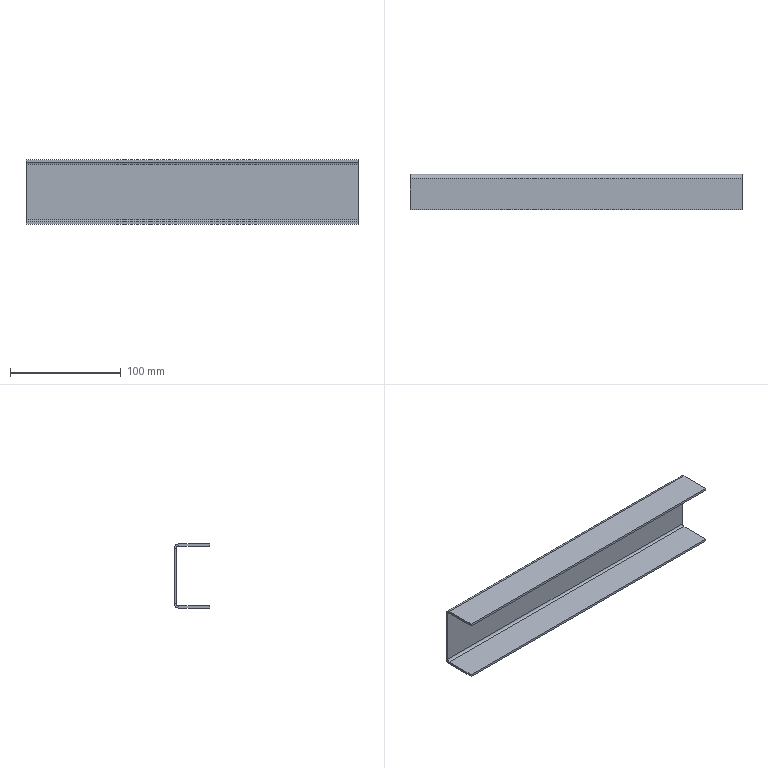Part | STEP file | JBJ-P-1007-04 | 1 solid | 22 faces | box 300 x 32 x 58 mm | volume 69255 mm3 | plane 18 | cylinder 4 | commonest cylinder face diameters 4 x2 8 x2
STEP:
#1=CARTESIAN_POINT('',(300.,28.,0.));
#2=VERTEX_POINT('',#1);
#3=CARTESIAN_POINT('',(300.,28.,2.));
#4=VERTEX_POINT('',#3);
#5=CARTESIAN_POINT('',(300.,28.,0.));
#6=DIRECTION('',(0.,0.,1.));
#7=VECTOR('',#6,1000.);
#8=LINE('',#5,#7);
#9=EDGE_CURVE('',#2,#4,#8,.T.);
#10=ORIENTED_EDGE('',*,*,#9,.F.);
#11=CARTESIAN_POINT('',(300.,30.,-2.));
#12=VERTEX_POINT('',#11);
#13=CARTESIAN_POINT('',(300.,28.,-2.));
#14=DIRECTION('',(-1.,0.,0.));
#15=DIRECTION('',(0.,0.,-1.));
#16=AXIS2_PLACEMENT_3D('',#13,#14,#15);
#17=CIRCLE('',#16,2.);
#18=EDGE_CURVE('',#2,#12,#17,.T.);
#19=ORIENTED_EDGE('',*,*,#18,.T.);
#20=CARTESIAN_POINT('',(300.,32.,-2.));
#21=VERTEX_POINT('',#20);
#22=CARTESIAN_POINT('',(300.,32.,-2.));
#23=DIRECTION('',(0.,-1.,0.));
#24=VECTOR('',#23,1000.);
#25=LINE('',#22,#24);
#26=EDGE_CURVE('',#21,#12,#25,.T.);
#27=ORIENTED_EDGE('',*,*,#26,.F.);
#28=CARTESIAN_POINT('',(300.,28.,-2.));
#29=DIRECTION('',(-1.,0.,0.));
#30=DIRECTION('',(0.,0.,-1.));
#31=AXIS2_PLACEMENT_3D('',#28,#29,#30);
#32=CIRCLE('',#31,4.);
#33=EDGE_CURVE('',#4,#21,#32,.T.);
#34=ORIENTED_EDGE('',*,*,#33,.F.);
#35=EDGE_LOOP('',(#10,#19,#27,#34));
#36=FACE_OUTER_BOUND('',#35,.T.);
#37=CARTESIAN_POINT('',(300.,28.,0.));
#38=DIRECTION('',(1.,0.,0.));
#39=DIRECTION('',(0.,0.,-1.));
#40=AXIS2_PLACEMENT_3D('',#37,#38,#39);
#41=PLANE('',#40);
#42=ADVANCED_FACE('',(#36),#41,.T.);
#43=CARTESIAN_POINT('',(300.,0.,0.));
#44=VERTEX_POINT('',#43);
#45=CARTESIAN_POINT('',(300.,0.,0.));
#46=DIRECTION('',(0.,1.,0.));
#47=VECTOR('',#46,1000.);
#48=LINE('',#45,#47);
#49=EDGE_CURVE('',#44,#2,#48,.T.);
#50=ORIENTED_EDGE('',*,*,#49,.T.);
#51=ORIENTED_EDGE('',*,*,#9,.T.);
#52=CARTESIAN_POINT('',(300.,0.,2.));
#53=VERTEX_POINT('',#52);
#54=CARTESIAN_POINT('',(300.,0.,2.));
#55=DIRECTION('',(0.,1.,0.));
#56=VECTOR('',#55,1000.);
#57=LINE('',#54,#56);
#58=EDGE_CURVE('',#53,#4,#57,.T.);
#59=ORIENTED_EDGE('',*,*,#58,.F.);
#60=CARTESIAN_POINT('',(300.,0.,0.));
#61=DIRECTION('',(0.,0.,1.));
#62=VECTOR('',#61,1000.);
#63=LINE('',#60,#62);
#64=EDGE_CURVE('',#44,#53,#63,.T.);
#65=ORIENTED_EDGE('',*,*,#64,.F.);
#66=EDGE_LOOP('',(#50,#51,#59,#65));
#67=FACE_OUTER_BOUND('',#66,.T.);
#68=CARTESIAN_POINT('',(300.,32.,-2.));
#69=DIRECTION('',(1.,0.,0.));
#70=DIRECTION('',(0.,0.,-1.));
#71=AXIS2_PLACEMENT_3D('',#68,#69,#70);
#72=PLANE('',#71);
#73=ADVANCED_FACE('',(#67),#72,.T.);
#74=CARTESIAN_POINT('',(0.,30.,-2.));
#75=VERTEX_POINT('',#74);
#76=CARTESIAN_POINT('',(0.,32.,-2.));
#77=VERTEX_POINT('',#76);
#78=CARTESIAN_POINT('',(0.,30.,-2.));
#79=DIRECTION('',(0.,1.,0.));
#80=VECTOR('',#79,1000.);
#81=LINE('',#78,#80);
#82=EDGE_CURVE('',#75,#77,#81,.T.);
#83=ORIENTED_EDGE('',*,*,#82,.F.);
#84=CARTESIAN_POINT('',(0.,28.,0.));
#85=VERTEX_POINT('',#84);
#86=CARTESIAN_POINT('',(0.,28.,-2.));
#87=DIRECTION('',(-1.,0.,0.));
#88=DIRECTION('',(0.,0.,-1.));
#89=AXIS2_PLACEMENT_3D('',#86,#87,#88);
#90=CIRCLE('',#89,2.);
#91=EDGE_CURVE('',#85,#75,#90,.T.);
#92=ORIENTED_EDGE('',*,*,#91,.F.);
#93=CARTESIAN_POINT('',(0.,28.,2.));
#94=VERTEX_POINT('',#93);
#95=CARTESIAN_POINT('',(0.,28.,2.));
#96=DIRECTION('',(0.,0.,-1.));
#97=VECTOR('',#96,1000.);
#98=LINE('',#95,#97);
#99=EDGE_CURVE('',#94,#85,#98,.T.);
#100=ORIENTED_EDGE('',*,*,#99,.F.);
#101=CARTESIAN_POINT('',(0.,28.,-2.));
#102=DIRECTION('',(-1.,0.,0.));
#103=DIRECTION('',(0.,0.,-1.));
#104=AXIS2_PLACEMENT_3D('',#101,#102,#103);
#105=CIRCLE('',#104,4.);
#106=EDGE_CURVE('',#94,#77,#105,.T.);
#107=ORIENTED_EDGE('',*,*,#106,.T.);
#108=EDGE_LOOP('',(#83,#92,#100,#107));
#109=FACE_OUTER_BOUND('',#108,.T.);
#110=CARTESIAN_POINT('',(0.,30.,-2.));
#111=DIRECTION('',(-1.,0.,0.));
#112=DIRECTION('',(0.,0.,1.));
#113=AXIS2_PLACEMENT_3D('',#110,#111,#112);
#114=PLANE('',#113);
#115=ADVANCED_FACE('',(#109),#114,.T.);
#116=CARTESIAN_POINT('',(0.,30.,-52.));
#117=VERTEX_POINT('',#116);
#118=CARTESIAN_POINT('',(0.,30.,0.));
#119=DIRECTION('',(0.,0.,-1.));
#120=VECTOR('',#119,1000.);
#121=LINE('',#118,#120);
#122=EDGE_CURVE('',#75,#117,#121,.T.);
#123=ORIENTED_EDGE('',*,*,#122,.F.);
#124=ORIENTED_EDGE('',*,*,#82,.T.);
#125=CARTESIAN_POINT('',(0.,32.,-52.));
#126=VERTEX_POINT('',#125);
#127=CARTESIAN_POINT('',(0.,32.,0.));
#128=DIRECTION('',(0.,0.,-1.));
#129=VECTOR('',#128,1000.);
#130=LINE('',#127,#129);
#131=EDGE_CURVE('',#77,#126,#130,.T.);
#132=ORIENTED_EDGE('',*,*,#131,.T.);
#133=CARTESIAN_POINT('',(0.,32.,-52.));
#134=DIRECTION('',(0.,-1.,0.));
#135=VECTOR('',#134,1000.);
#136=LINE('',#133,#135);
#137=EDGE_CURVE('',#126,#117,#136,.T.);
#138=ORIENTED_EDGE('',*,*,#137,.T.);
#139=EDGE_LOOP('',(#123,#124,#132,#138));
#140=FACE_OUTER_BOUND('',#139,.T.);
#141=CARTESIAN_POINT('',(0.,28.,2.));
#142=DIRECTION('',(-1.,0.,0.));
#143=DIRECTION('',(0.,0.,1.));
#144=AXIS2_PLACEMENT_3D('',#141,#142,#143);
#145=PLANE('',#144);
#146=ADVANCED_FACE('',(#140),#145,.T.);
#147=CARTESIAN_POINT('',(300.,30.,-52.));
#148=VERTEX_POINT('',#147);
#149=CARTESIAN_POINT('',(300.,32.,-52.));
#150=VERTEX_POINT('',#149);
#151=CARTESIAN_POINT('',(300.,30.,-52.));
#152=DIRECTION('',(0.,1.,0.));
#153=VECTOR('',#152,1000.);
#154=LINE('',#151,#153);
#155=EDGE_CURVE('',#148,#150,#154,.T.);
#156=ORIENTED_EDGE('',*,*,#155,.F.);
#157=CARTESIAN_POINT('',(300.,28.,-54.));
#158=VERTEX_POINT('',#157);
#159=CARTESIAN_POINT('',(300.,28.,-52.));
#160=DIRECTION('',(-1.,0.,0.));
#161=DIRECTION('',(0.,0.,-1.));
#162=AXIS2_PLACEMENT_3D('',#159,#160,#161);
#163=CIRCLE('',#162,2.);
#164=EDGE_CURVE('',#148,#158,#163,.T.);
#165=ORIENTED_EDGE('',*,*,#164,.T.);
#166=CARTESIAN_POINT('',(300.,28.,-56.));
#167=VERTEX_POINT('',#166);
#168=CARTESIAN_POINT('',(300.,28.,-56.));
#169=DIRECTION('',(0.,0.,1.));
#170=VECTOR('',#169,1000.);
#171=LINE('',#168,#170);
#172=EDGE_CURVE('',#167,#158,#171,.T.);
#173=ORIENTED_EDGE('',*,*,#172,.F.);
#174=CARTESIAN_POINT('',(300.,28.,-52.));
#175=DIRECTION('',(-1.,0.,0.));
#176=DIRECTION('',(0.,0.,-1.));
#177=AXIS2_PLACEMENT_3D('',#174,#175,#176);
#178=CIRCLE('',#177,4.);
#179=EDGE_CURVE('',#150,#167,#178,.T.);
#180=ORIENTED_EDGE('',*,*,#179,.F.);
#181=EDGE_LOOP('',(#156,#165,#173,#180));
#182=FACE_OUTER_BOUND('',#181,.T.);
#183=CARTESIAN_POINT('',(300.,30.,-52.));
#184=DIRECTION('',(1.,0.,0.));
#185=DIRECTION('',(0.,0.,-1.));
#186=AXIS2_PLACEMENT_3D('',#183,#184,#185);
#187=PLANE('',#186);
#188=ADVANCED_FACE('',(#182),#187,.T.);
#189=CARTESIAN_POINT('',(300.,30.,0.));
#190=DIRECTION('',(0.,0.,-1.));
#191=VECTOR('',#190,1000.);
#192=LINE('',#189,#191);
#193=EDGE_CURVE('',#12,#148,#192,.T.);
#194=ORIENTED_EDGE('',*,*,#193,.T.);
#195=ORIENTED_EDGE('',*,*,#155,.T.);
#196=CARTESIAN_POINT('',(300.,32.,0.));
#197=DIRECTION('',(0.,0.,-1.));
#198=VECTOR('',#197,1000.);
#199=LINE('',#196,#198);
#200=EDGE_CURVE('',#21,#150,#199,.T.);
#201=ORIENTED_EDGE('',*,*,#200,.F.);
#202=ORIENTED_EDGE('',*,*,#26,.T.);
#203=EDGE_LOOP('',(#194,#195,#201,#202));
#204=FACE_OUTER_BOUND('',#203,.T.);
#205=CARTESIAN_POINT('',(300.,28.,-56.));
#206=DIRECTION('',(1.,0.,0.));
#207=DIRECTION('',(0.,0.,-1.));
#208=AXIS2_PLACEMENT_3D('',#205,#206,#207);
#209=PLANE('',#208);
#210=ADVANCED_FACE('',(#204),#209,.T.);
#211=CARTESIAN_POINT('',(0.,28.,-54.));
#212=VERTEX_POINT('',#211);
#213=CARTESIAN_POINT('',(0.,28.,-56.));
#214=VERTEX_POINT('',#213);
#215=CARTESIAN_POINT('',(0.,28.,-54.));
#216=DIRECTION('',(0.,0.,-1.));
#217=VECTOR('',#216,1000.);
#218=LINE('',#215,#217);
#219=EDGE_CURVE('',#212,#214,#218,.T.);
#220=ORIENTED_EDGE('',*,*,#219,.F.);
#221=CARTESIAN_POINT('',(0.,28.,-52.));
#222=DIRECTION('',(-1.,0.,0.));
#223=DIRECTION('',(0.,0.,-1.));
#224=AXIS2_PLACEMENT_3D('',#221,#222,#223);
#225=CIRCLE('',#224,2.);
#226=EDGE_CURVE('',#117,#212,#225,.T.);
#227=ORIENTED_EDGE('',*,*,#226,.F.);
#228=ORIENTED_EDGE('',*,*,#137,.F.);
#229=CARTESIAN_POINT('',(0.,28.,-52.));
#230=DIRECTION('',(-1.,0.,0.));
#231=DIRECTION('',(0.,0.,-1.));
#232=AXIS2_PLACEMENT_3D('',#229,#230,#231);
#233=CIRCLE('',#232,4.);
#234=EDGE_CURVE('',#126,#214,#233,.T.);
#235=ORIENTED_EDGE('',*,*,#234,.T.);
#236=EDGE_LOOP('',(#220,#227,#228,#235));
#237=FACE_OUTER_BOUND('',#236,.T.);
#238=CARTESIAN_POINT('',(0.,28.,-54.));
#239=DIRECTION('',(-1.,0.,0.));
#240=DIRECTION('',(0.,0.,1.));
#241=AXIS2_PLACEMENT_3D('',#238,#239,#240);
#242=PLANE('',#241);
#243=ADVANCED_FACE('',(#237),#242,.T.);
#244=CARTESIAN_POINT('',(0.,0.,-54.));
#245=VERTEX_POINT('',#244);
#246=CARTESIAN_POINT('',(0.,30.,-54.));
#247=DIRECTION('',(0.,-1.,0.));
#248=VECTOR('',#247,1000.);
#249=LINE('',#246,#248);
#250=EDGE_CURVE('',#212,#245,#249,.T.);
#251=ORIENTED_EDGE('',*,*,#250,.F.);
#252=ORIENTED_EDGE('',*,*,#219,.T.);
#253=CARTESIAN_POINT('',(0.,0.,-56.));
#254=VERTEX_POINT('',#253);
#255=CARTESIAN_POINT('',(0.,30.,-56.));
#256=DIRECTION('',(0.,-1.,0.));
#257=VECTOR('',#256,1000.);
#258=LINE('',#255,#257);
#259=EDGE_CURVE('',#214,#254,#258,.T.);
#260=ORIENTED_EDGE('',*,*,#259,.T.);
#261=CARTESIAN_POINT('',(0.,0.,-56.));
#262=DIRECTION('',(0.,0.,1.));
#263=VECTOR('',#262,1000.);
#264=LINE('',#261,#263);
#265=EDGE_CURVE('',#254,#245,#264,.T.);
#266=ORIENTED_EDGE('',*,*,#265,.T.);
#267=EDGE_LOOP('',(#251,#252,#260,#266));
#268=FACE_OUTER_BOUND('',#267,.T.);
#269=CARTESIAN_POINT('',(0.,32.,-52.));
#270=DIRECTION('',(-1.,0.,0.));
#271=DIRECTION('',(0.,0.,1.));
#272=AXIS2_PLACEMENT_3D('',#269,#270,#271);
#273=PLANE('',#272);
#274=ADVANCED_FACE('',(#268),#273,.T.);
#275=ORIENTED_EDGE('',*,*,#250,.T.);
#276=CARTESIAN_POINT('',(300.,0.,-54.));
#277=VERTEX_POINT('',#276);
#278=CARTESIAN_POINT('',(300.,0.,-54.));
#279=DIRECTION('',(-1.,0.,0.));
#280=VECTOR('',#279,1000.);
#281=LINE('',#278,#280);
#282=EDGE_CURVE('',#277,#245,#281,.T.);
#283=ORIENTED_EDGE('',*,*,#282,.F.);
#284=CARTESIAN_POINT('',(300.,30.,-54.));
#285=DIRECTION('',(0.,-1.,0.));
#286=VECTOR('',#285,1000.);
#287=LINE('',#284,#286);
#288=EDGE_CURVE('',#158,#277,#287,.T.);
#289=ORIENTED_EDGE('',*,*,#288,.F.);
#290=CARTESIAN_POINT('',(300.,28.,-54.));
#291=DIRECTION('',(-1.,0.,0.));
#292=VECTOR('',#291,1000.);
#293=LINE('',#290,#292);
#294=EDGE_CURVE('',#158,#212,#293,.T.);
#295=ORIENTED_EDGE('',*,*,#294,.T.);
#296=EDGE_LOOP('',(#275,#283,#289,#295));
#297=FACE_OUTER_BOUND('',#296,.T.);
#298=CARTESIAN_POINT('',(300.,30.,-54.));
#299=DIRECTION('',(0.,0.,-1.));
#300=DIRECTION('',(-1.,0.,0.));
#301=AXIS2_PLACEMENT_3D('',#298,#299,#300);
#302=PLANE('',#301);
#303=ADVANCED_FACE('',(#297),#302,.F.);
#304=ORIENTED_EDGE('',*,*,#265,.F.);
#305=CARTESIAN_POINT('',(300.,0.,-56.));
#306=VERTEX_POINT('',#305);
#307=CARTESIAN_POINT('',(300.,0.,-56.));
#308=DIRECTION('',(-1.,0.,0.));
#309=VECTOR('',#308,1000.);
#310=LINE('',#307,#309);
#311=EDGE_CURVE('',#306,#254,#310,.T.);
#312=ORIENTED_EDGE('',*,*,#311,.F.);
#313=CARTESIAN_POINT('',(300.,0.,-56.));
#314=DIRECTION('',(0.,0.,1.));
#315=VECTOR('',#314,1000.);
#316=LINE('',#313,#315);
#317=EDGE_CURVE('',#306,#277,#316,.T.);
#318=ORIENTED_EDGE('',*,*,#317,.T.);
#319=ORIENTED_EDGE('',*,*,#282,.T.);
#320=EDGE_LOOP('',(#304,#312,#318,#319));
#321=FACE_OUTER_BOUND('',#320,.T.);
#322=CARTESIAN_POINT('',(300.,0.,-56.));
#323=DIRECTION('',(0.,-1.,0.));
#324=DIRECTION('',(0.,0.,-1.));
#325=AXIS2_PLACEMENT_3D('',#322,#323,#324);
#326=PLANE('',#325);
#327=ADVANCED_FACE('',(#321),#326,.T.);
#328=ORIENTED_EDGE('',*,*,#259,.F.);
#329=CARTESIAN_POINT('',(300.,28.,-56.));
#330=DIRECTION('',(-1.,0.,0.));
#331=VECTOR('',#330,1000.);
#332=LINE('',#329,#331);
#333=EDGE_CURVE('',#167,#214,#332,.T.);
#334=ORIENTED_EDGE('',*,*,#333,.F.);
#335=CARTESIAN_POINT('',(300.,30.,-56.));
#336=DIRECTION('',(0.,-1.,0.));
#337=VECTOR('',#336,1000.);
#338=LINE('',#335,#337);
#339=EDGE_CURVE('',#167,#306,#338,.T.);
#340=ORIENTED_EDGE('',*,*,#339,.T.);
#341=ORIENTED_EDGE('',*,*,#311,.T.);
#342=EDGE_LOOP('',(#328,#334,#340,#341));
#343=FACE_OUTER_BOUND('',#342,.T.);
#344=CARTESIAN_POINT('',(300.,30.,-56.));
#345=DIRECTION('',(0.,0.,-1.));
#346=DIRECTION('',(-1.,0.,0.));
#347=AXIS2_PLACEMENT_3D('',#344,#345,#346);
#348=PLANE('',#347);
#349=ADVANCED_FACE('',(#343),#348,.T.);
#350=ORIENTED_EDGE('',*,*,#234,.F.);
#351=CARTESIAN_POINT('',(300.,32.,-52.));
#352=DIRECTION('',(-1.,0.,0.));
#353=VECTOR('',#352,1000.);
#354=LINE('',#351,#353);
#355=EDGE_CURVE('',#150,#126,#354,.T.);
#356=ORIENTED_EDGE('',*,*,#355,.F.);
#357=ORIENTED_EDGE('',*,*,#179,.T.);
#358=ORIENTED_EDGE('',*,*,#333,.T.);
#359=EDGE_LOOP('',(#350,#356,#357,#358));
#360=FACE_OUTER_BOUND('',#359,.T.);
#361=CARTESIAN_POINT('',(300.,28.,-52.));
#362=DIRECTION('',(-1.,0.,0.));
#363=DIRECTION('',(0.,0.,1.));
#364=AXIS2_PLACEMENT_3D('',#361,#362,#363);
#365=CYLINDRICAL_SURFACE('',#364,4.);
#366=ADVANCED_FACE('',(#360),#365,.T.);
#367=ORIENTED_EDGE('',*,*,#131,.F.);
#368=CARTESIAN_POINT('',(300.,32.,-2.));
#369=DIRECTION('',(-1.,0.,0.));
#370=VECTOR('',#369,1000.);
#371=LINE('',#368,#370);
#372=EDGE_CURVE('',#21,#77,#371,.T.);
#373=ORIENTED_EDGE('',*,*,#372,.F.);
#374=ORIENTED_EDGE('',*,*,#200,.T.);
#375=ORIENTED_EDGE('',*,*,#355,.T.);
#376=EDGE_LOOP('',(#367,#373,#374,#375));
#377=FACE_OUTER_BOUND('',#376,.T.);
#378=CARTESIAN_POINT('',(300.,32.,0.));
#379=DIRECTION('',(0.,1.,0.));
#380=DIRECTION('',(0.,0.,1.));
#381=AXIS2_PLACEMENT_3D('',#378,#379,#380);
#382=PLANE('',#381);
#383=ADVANCED_FACE('',(#377),#382,.T.);
#384=ORIENTED_EDGE('',*,*,#106,.F.);
#385=CARTESIAN_POINT('',(300.,28.,2.));
#386=DIRECTION('',(-1.,0.,0.));
#387=VECTOR('',#386,1000.);
#388=LINE('',#385,#387);
#389=EDGE_CURVE('',#4,#94,#388,.T.);
#390=ORIENTED_EDGE('',*,*,#389,.F.);
#391=ORIENTED_EDGE('',*,*,#33,.T.);
#392=ORIENTED_EDGE('',*,*,#372,.T.);
#393=EDGE_LOOP('',(#384,#390,#391,#392));
#394=FACE_OUTER_BOUND('',#393,.T.);
#395=CARTESIAN_POINT('',(300.,28.,-2.));
#396=DIRECTION('',(-1.,0.,0.));
#397=DIRECTION('',(0.,0.,1.));
#398=AXIS2_PLACEMENT_3D('',#395,#396,#397);
#399=CYLINDRICAL_SURFACE('',#398,4.);
#400=ADVANCED_FACE('',(#394),#399,.T.);
#401=CARTESIAN_POINT('',(0.,0.,2.));
#402=VERTEX_POINT('',#401);
#403=CARTESIAN_POINT('',(0.,0.,2.));
#404=DIRECTION('',(0.,1.,0.));
#405=VECTOR('',#404,1000.);
#406=LINE('',#403,#405);
#407=EDGE_CURVE('',#402,#94,#406,.T.);
#408=ORIENTED_EDGE('',*,*,#407,.F.);
#409=CARTESIAN_POINT('',(300.,0.,2.));
#410=DIRECTION('',(-1.,0.,0.));
#411=VECTOR('',#410,1000.);
#412=LINE('',#409,#411);
#413=EDGE_CURVE('',#53,#402,#412,.T.);
#414=ORIENTED_EDGE('',*,*,#413,.F.);
#415=ORIENTED_EDGE('',*,*,#58,.T.);
#416=ORIENTED_EDGE('',*,*,#389,.T.);
#417=EDGE_LOOP('',(#408,#414,#415,#416));
#418=FACE_OUTER_BOUND('',#417,.T.);
#419=CARTESIAN_POINT('',(300.,0.,2.));
#420=DIRECTION('',(0.,0.,1.));
#421=DIRECTION('',(1.,0.,0.));
#422=AXIS2_PLACEMENT_3D('',#419,#420,#421);
#423=PLANE('',#422);
#424=ADVANCED_FACE('',(#418),#423,.T.);
#425=CARTESIAN_POINT('',(0.,0.,0.));
#426=VERTEX_POINT('',#425);
#427=CARTESIAN_POINT('',(0.,0.,0.));
#428=DIRECTION('',(0.,0.,1.));
#429=VECTOR('',#428,1000.);
#430=LINE('',#427,#429);
#431=EDGE_CURVE('',#426,#402,#430,.T.);
#432=ORIENTED_EDGE('',*,*,#431,.F.);
#433=CARTESIAN_POINT('',(300.,0.,0.));
#434=DIRECTION('',(-1.,0.,0.));
#435=VECTOR('',#434,1000.);
#436=LINE('',#433,#435);
#437=EDGE_CURVE('',#44,#426,#436,.T.);
#438=ORIENTED_EDGE('',*,*,#437,.F.);
#439=ORIENTED_EDGE('',*,*,#64,.T.);
#440=ORIENTED_EDGE('',*,*,#413,.T.);
#441=EDGE_LOOP('',(#432,#438,#439,#440));
#442=FACE_OUTER_BOUND('',#441,.T.);
#443=CARTESIAN_POINT('',(300.,0.,0.));
#444=DIRECTION('',(0.,-1.,0.));
#445=DIRECTION('',(0.,0.,-1.));
#446=AXIS2_PLACEMENT_3D('',#443,#444,#445);
#447=PLANE('',#446);
#448=ADVANCED_FACE('',(#442),#447,.T.);
#449=CARTESIAN_POINT('',(0.,0.,0.));
#450=DIRECTION('',(0.,1.,0.));
#451=VECTOR('',#450,1000.);
#452=LINE('',#449,#451);
#453=EDGE_CURVE('',#426,#85,#452,.T.);
#454=ORIENTED_EDGE('',*,*,#453,.T.);
#455=CARTESIAN_POINT('',(300.,28.,0.));
#456=DIRECTION('',(-1.,0.,0.));
#457=VECTOR('',#456,1000.);
#458=LINE('',#455,#457);
#459=EDGE_CURVE('',#2,#85,#458,.T.);
#460=ORIENTED_EDGE('',*,*,#459,.F.);
#461=ORIENTED_EDGE('',*,*,#49,.F.);
#462=ORIENTED_EDGE('',*,*,#437,.T.);
#463=EDGE_LOOP('',(#454,#460,#461,#462));
#464=FACE_OUTER_BOUND('',#463,.T.);
#465=CARTESIAN_POINT('',(300.,0.,0.));
#466=DIRECTION('',(0.,0.,1.));
#467=DIRECTION('',(1.,0.,0.));
#468=AXIS2_PLACEMENT_3D('',#465,#466,#467);
#469=PLANE('',#468);
#470=ADVANCED_FACE('',(#464),#469,.F.);
#471=ORIENTED_EDGE('',*,*,#91,.T.);
#472=CARTESIAN_POINT('',(300.,30.,-2.));
#473=DIRECTION('',(-1.,0.,0.));
#474=VECTOR('',#473,1000.);
#475=LINE('',#472,#474);
#476=EDGE_CURVE('',#12,#75,#475,.T.);
#477=ORIENTED_EDGE('',*,*,#476,.F.);
#478=ORIENTED_EDGE('',*,*,#18,.F.);
#479=ORIENTED_EDGE('',*,*,#459,.T.);
#480=EDGE_LOOP('',(#471,#477,#478,#479));
#481=FACE_OUTER_BOUND('',#480,.T.);
#482=CARTESIAN_POINT('',(300.,28.,-2.));
#483=DIRECTION('',(-1.,0.,0.));
#484=DIRECTION('',(0.,0.,1.));
#485=AXIS2_PLACEMENT_3D('',#482,#483,#484);
#486=CYLINDRICAL_SURFACE('',#485,2.);
#487=ADVANCED_FACE('',(#481),#486,.F.);
#488=ORIENTED_EDGE('',*,*,#122,.T.);
#489=CARTESIAN_POINT('',(300.,30.,-52.));
#490=DIRECTION('',(-1.,0.,0.));
#491=VECTOR('',#490,1000.);
#492=LINE('',#489,#491);
#493=EDGE_CURVE('',#148,#117,#492,.T.);
#494=ORIENTED_EDGE('',*,*,#493,.F.);
#495=ORIENTED_EDGE('',*,*,#193,.F.);
#496=ORIENTED_EDGE('',*,*,#476,.T.);
#497=EDGE_LOOP('',(#488,#494,#495,#496));
#498=FACE_OUTER_BOUND('',#497,.T.);
#499=CARTESIAN_POINT('',(300.,30.,0.));
#500=DIRECTION('',(0.,1.,0.));
#501=DIRECTION('',(0.,0.,1.));
#502=AXIS2_PLACEMENT_3D('',#499,#500,#501);
#503=PLANE('',#502);
#504=ADVANCED_FACE('',(#498),#503,.F.);
#505=ORIENTED_EDGE('',*,*,#226,.T.);
#506=ORIENTED_EDGE('',*,*,#294,.F.);
#507=ORIENTED_EDGE('',*,*,#164,.F.);
#508=ORIENTED_EDGE('',*,*,#493,.T.);
#509=EDGE_LOOP('',(#505,#506,#507,#508));
#510=FACE_OUTER_BOUND('',#509,.T.);
#511=CARTESIAN_POINT('',(300.,28.,-52.));
#512=DIRECTION('',(-1.,0.,0.));
#513=DIRECTION('',(0.,0.,1.));
#514=AXIS2_PLACEMENT_3D('',#511,#512,#513);
#515=CYLINDRICAL_SURFACE('',#514,2.);
#516=ADVANCED_FACE('',(#510),#515,.F.);
#517=ORIENTED_EDGE('',*,*,#288,.T.);
#518=ORIENTED_EDGE('',*,*,#317,.F.);
#519=ORIENTED_EDGE('',*,*,#339,.F.);
#520=ORIENTED_EDGE('',*,*,#172,.T.);
#521=EDGE_LOOP('',(#517,#518,#519,#520));
#522=FACE_OUTER_BOUND('',#521,.T.);
#523=CARTESIAN_POINT('',(300.,28.,-52.));
#524=DIRECTION('',(1.,0.,0.));
#525=DIRECTION('',(0.,0.,-1.));
#526=AXIS2_PLACEMENT_3D('',#523,#524,#525);
#527=PLANE('',#526);
#528=ADVANCED_FACE('',(#522),#527,.T.);
#529=ORIENTED_EDGE('',*,*,#407,.T.);
#530=ORIENTED_EDGE('',*,*,#99,.T.);
#531=ORIENTED_EDGE('',*,*,#453,.F.);
#532=ORIENTED_EDGE('',*,*,#431,.T.);
#533=EDGE_LOOP('',(#529,#530,#531,#532));
#534=FACE_OUTER_BOUND('',#533,.T.);
#535=CARTESIAN_POINT('',(0.,28.,-52.));
#536=DIRECTION('',(1.,0.,0.));
#537=DIRECTION('',(0.,0.,-1.));
#538=AXIS2_PLACEMENT_3D('',#535,#536,#537);
#539=PLANE('',#538);
#540=ADVANCED_FACE('',(#534),#539,.F.);
#541=CLOSED_SHELL('',(#42,#73,#115,#146,#188,#210,#243,#274,#303,#327,#349,#366,#383,#400,#424,#448,#470,#487,#504,#516,#528,#540));
#542=MANIFOLD_SOLID_BREP('',#541);
#543=CARTESIAN_POINT('',(0.,0.,0.));
#544=DIRECTION('',(0.,0.,1.));
#545=DIRECTION('',(1.,0.,0.));
#546=AXIS2_PLACEMENT_3D('',#543,#544,#545);
#547=(LENGTH_UNIT()NAMED_UNIT(*)SI_UNIT(.MILLI.,.METRE.));
#548=UNCERTAINTY_MEASURE_WITH_UNIT(LENGTH_MEASURE(0.00001),#547,'','');
#549=(NAMED_UNIT(*)PLANE_ANGLE_UNIT()SI_UNIT($,.RADIAN.));
#550=(NAMED_UNIT(*)SI_UNIT($,.STERADIAN.)SOLID_ANGLE_UNIT());
#551=(GEOMETRIC_REPRESENTATION_CONTEXT(3)GLOBAL_UNCERTAINTY_ASSIGNED_CONTEXT((#548))GLOBAL_UNIT_ASSIGNED_CONTEXT((#547,#549,#550))REPRESENTATION_CONTEXT('',''));
#552=ADVANCED_BREP_SHAPE_REPRESENTATION('',(#542,#546),#551);